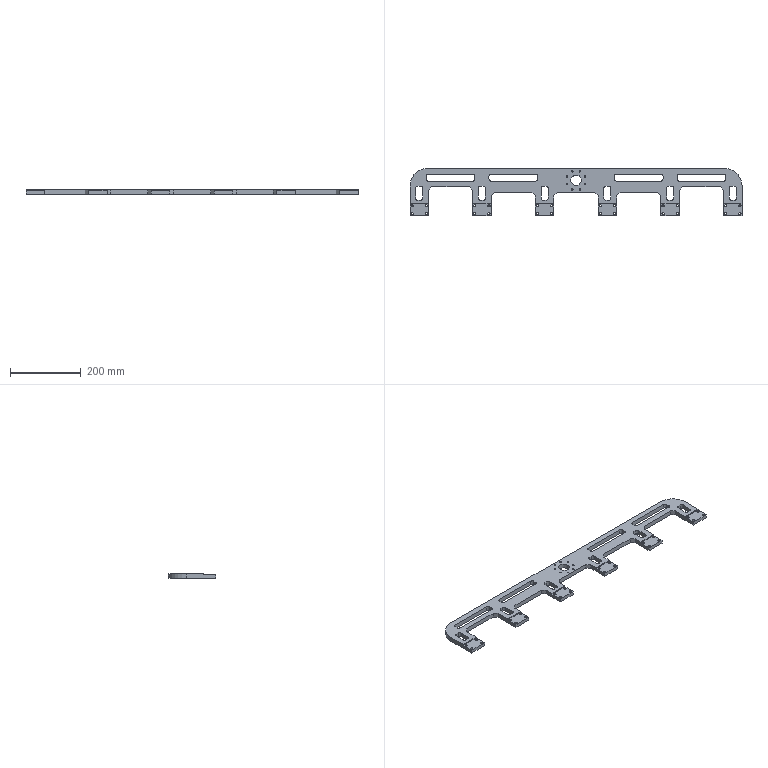CAM job | NX | 3-axis milling, drilling | part box 941 x 134 x 13 mm | stock box 945 x 138 x 15 mm
Tools:
number,name,description,diameter,corner_radius,flute_length,length,flutes
1,D63,Milling Tool-5 Parameters,63.0,0.0,50.0,75.0,2
7,D6A45,Milling Tool-5 Parameters,6.0,0.0,50.0,75.0,2
14,4.5ZT,Drilling Tool,4.5,0.0,35.0,50.0,2
15,6.5ZT,Drilling Tool,6.5,0.0,35.0,50.0,2
10,D10,Milling Tool-5 Parameters,10.0,0.0,50.0,75.0,2
Operations:
program,operation,operation_type,tool,method,geometry_group,spindle_rpm,surface_speed,feed_per_tooth,feed_cut,feed_plunge,cut_length_mm,path_length_mm,cut_time_min,machine_time_min
1,FLOOR_WALL_COPY,VolumeBased25DMillingOperation,D63,METHOD,A,6500.0,1286.0,0.1154,1500.0,100.0,3555.532,3609.532,2.37,2.376
1,DRILLING_COPY_1,Operation,D6A45,METHOD,A,5000.0,94.0,0.025,250.0,0.0,84.0,1071.375,0.336,0.4347
1,DRILLING_COPY_COPY_1,Operation,4.5ZT,METHOD,A,2000.0,28.0,0.0625,250.0,0.0,146.815,526.106,0.5873,0.6252
1,DRILLING_COPY_COPY_COPY,Operation,6.5ZT,METHOD,A,2000.0,28.0,0.0625,250.0,0.0,227.434,1078.836,0.9097,0.9949
1,ZLEVEL_PROFILE_COPY_3,ZLevelMilling,D10,METHOD,A,9500.0,298.0,0.1842,3500.0,1000.0,22472.277,23374.777,6.516,6.606
1,ZLEVEL_PROFILE_COPY_3_COPY,ZLevelMilling,D10,METHOD,A,9500.0,298.0,0.0632,1200.0,1000.0,1604.9,1681.9,1.339,1.347
1,ZLEVEL_PROFILE_COPY_2_COPY_COPY,ZLevelMilling,D10,METHOD,A,9500.0,298.0,0.1053,2000.0,1000.0,511.815,582.315,0.2795,0.2865
1,ZLEVEL_PROFILE_COPY_2_COPY,ZLevelMilling,D10,METHOD,A,9500.0,298.0,0.1842,3500.0,1000.0,12396.805,14015.322,3.744,3.906
1,ZLEVEL_PROFILE_COPY_COPY_1,ZLevelMilling,D10,METHOD,A,9500.0,298.0,0.0789,1500.0,1000.0,3448.978,4562.78,2.386,2.497
1,FLOOR_WALL_1_COPY_1,VolumeBased25DMillingOperation,D10,METHOD,A,9500.0,298.0,0.1579,3000.0,1000.0,4586.35,5222.341,1.544,1.608
1,FLOOR_WALL_1_COPY_COPY,VolumeBased25DMillingOperation,D10,METHOD,A,9500.0,298.0,0.0789,1500.0,1000.0,1254.257,1848.072,0.8413,0.9006
1,PLANAR_MILL_COPY_1,PlanarMilling,D6A45,METHOD,A,9500.0,179.0,0.0737,1400.0,100.0,2497.387,4153.666,1.784,1.95
1,PLANAR_MILL_COPY_COPY,PlanarMilling,D6A45,METHOD,A,9500.0,179.0,0.0737,1400.0,100.0,599.066,2778.071,0.4279,0.6458
2,FLOOR_WALL_COPY_COPY,VolumeBased25DMillingOperation,D63,METHOD,A,6500.0,1286.0,0.1154,1500.0,100.0,2858.46,2912.46,1.906,1.911
2,DRILLING_COPY_1_COPY,Operation,D6A45,METHOD,A,5000.0,94.0,0.025,250.0,0.0,48.0,719.969,0.192,0.2592
2,DRILLING_COPY_COPY_COPY_COPY,Operation,6.5ZT,METHOD,A,2000.0,28.0,0.0625,250.0,0.0,227.434,1078.836,0.9097,0.9949
2,ZLEVEL_PROFILE_COPY_3_COPY_1,ZLevelMilling,D10,METHOD,A,9500.0,298.0,0.1842,3500.0,1000.0,18399.753,19302.253,5.363,5.453
2,ZLEVEL_PROFILE_COPY_3_COPY_COPY,ZLevelMilling,D10,METHOD,A,9500.0,298.0,0.0632,1200.0,1000.0,1314.175,1391.175,1.097,1.104
2,ZLEVEL_PROFILE_COPY_2_COPY_COPY_1,ZLevelMilling,D10,METHOD,A,9500.0,298.0,0.1842,3500.0,1000.0,11430.87,12540.961,3.434,3.545
2,ZLEVEL_PROFILE_COPY_COPY_1_COPY,ZLevelMilling,D10,METHOD,A,9500.0,298.0,0.0789,1500.0,1000.0,3166.761,4131.694,2.183,2.28
2,FLOOR_WALL_1_COPY_1_COPY,VolumeBased25DMillingOperation,D10,METHOD,A,9500.0,298.0,0.1579,3000.0,1000.0,4586.35,5229.24,1.544,1.608
2,FLOOR_WALL_1_COPY_COPY_COPY,VolumeBased25DMillingOperation,D10,METHOD,A,9500.0,298.0,0.0789,1500.0,1000.0,1254.257,1848.072,0.8413,0.9006
2,PLANAR_MILL_COPY_1_COPY,PlanarMilling,D6A45,METHOD,A,9500.0,179.0,0.0737,1400.0,100.0,2026.337,3235.613,1.447,1.568
2,PLANAR_MILL_COPY_COPY_COPY,PlanarMilling,D6A45,METHOD,A,9500.0,179.0,0.0737,1400.0,100.0,599.066,2807.127,0.4279,0.6487